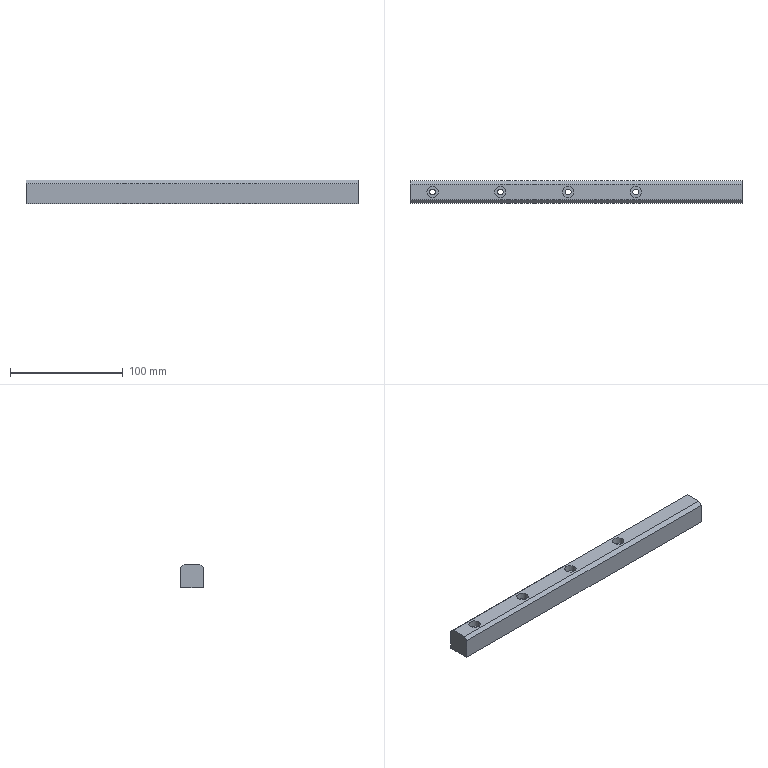Part | NX | 1 solid | 20 faces | box 294 x 20 x 21 mm | volume 117693 mm3 | plane 12 | cylinder 8 | commonest cylinder face diameters 5.3 x4 10 x4
STEP:
#1=CARTESIAN_POINT('',(-124.35,0.,0.));
#2=VERTEX_POINT('',#1);
#3=CARTESIAN_POINT('',(-127.,0.,0.));
#4=DIRECTION('',(0.,0.,1.));
#5=DIRECTION('',(1.,0.,0.));
#6=AXIS2_PLACEMENT_3D('',#3,#4,#5);
#7=CIRCLE('',#6,2.65);
#8=EDGE_CURVE('',#2,#2,#7,.T.);
#9=ORIENTED_EDGE('',*,*,#8,.F.);
#10=EDGE_LOOP('',(#9));
#11=FACE_BOUND('',#10,.T.);
#12=CARTESIAN_POINT('',(-124.35,0.,15.3));
#13=VERTEX_POINT('',#12);
#14=CARTESIAN_POINT('',(-127.,0.,15.3));
#15=DIRECTION('',(0.,0.,1.));
#16=DIRECTION('',(1.,0.,0.));
#17=AXIS2_PLACEMENT_3D('',#14,#15,#16);
#18=CIRCLE('',#17,2.65);
#19=EDGE_CURVE('',#13,#13,#18,.T.);
#20=ORIENTED_EDGE('',*,*,#19,.T.);
#21=EDGE_LOOP('',(#20));
#22=FACE_BOUND('',#21,.T.);
#23=CARTESIAN_POINT('',(-127.,0.,294.));
#24=DIRECTION('',(0.,0.,-1.));
#25=DIRECTION('',(1.,0.,0.));
#26=AXIS2_PLACEMENT_3D('',#23,#24,#25);
#27=CYLINDRICAL_SURFACE('',#26,2.65);
#28=ADVANCED_FACE('',(#11,#22),#27,.F.);
#29=CARTESIAN_POINT('',(-64.35,0.,0.));
#30=VERTEX_POINT('',#29);
#31=CARTESIAN_POINT('',(-67.,0.,0.));
#32=DIRECTION('',(0.,0.,1.));
#33=DIRECTION('',(1.,0.,0.));
#34=AXIS2_PLACEMENT_3D('',#31,#32,#33);
#35=CIRCLE('',#34,2.65);
#36=EDGE_CURVE('',#30,#30,#35,.T.);
#37=ORIENTED_EDGE('',*,*,#36,.F.);
#38=EDGE_LOOP('',(#37));
#39=FACE_BOUND('',#38,.T.);
#40=CARTESIAN_POINT('',(-64.35,0.,15.3));
#41=VERTEX_POINT('',#40);
#42=CARTESIAN_POINT('',(-67.,0.,15.3));
#43=DIRECTION('',(0.,0.,1.));
#44=DIRECTION('',(1.,0.,0.));
#45=AXIS2_PLACEMENT_3D('',#42,#43,#44);
#46=CIRCLE('',#45,2.65);
#47=EDGE_CURVE('',#41,#41,#46,.T.);
#48=ORIENTED_EDGE('',*,*,#47,.T.);
#49=EDGE_LOOP('',(#48));
#50=FACE_BOUND('',#49,.T.);
#51=CARTESIAN_POINT('',(-67.,0.,294.));
#52=DIRECTION('',(0.,0.,-1.));
#53=DIRECTION('',(1.,0.,0.));
#54=AXIS2_PLACEMENT_3D('',#51,#52,#53);
#55=CYLINDRICAL_SURFACE('',#54,2.65);
#56=ADVANCED_FACE('',(#39,#50),#55,.F.);
#57=CARTESIAN_POINT('',(-4.35,0.,0.));
#58=VERTEX_POINT('',#57);
#59=CARTESIAN_POINT('',(-7.,0.,0.));
#60=DIRECTION('',(0.,0.,1.));
#61=DIRECTION('',(1.,0.,0.));
#62=AXIS2_PLACEMENT_3D('',#59,#60,#61);
#63=CIRCLE('',#62,2.65);
#64=EDGE_CURVE('',#58,#58,#63,.T.);
#65=ORIENTED_EDGE('',*,*,#64,.F.);
#66=EDGE_LOOP('',(#65));
#67=FACE_BOUND('',#66,.T.);
#68=CARTESIAN_POINT('',(-4.35,0.,15.3));
#69=VERTEX_POINT('',#68);
#70=CARTESIAN_POINT('',(-7.,0.,15.3));
#71=DIRECTION('',(0.,0.,1.));
#72=DIRECTION('',(1.,0.,0.));
#73=AXIS2_PLACEMENT_3D('',#70,#71,#72);
#74=CIRCLE('',#73,2.65);
#75=EDGE_CURVE('',#69,#69,#74,.T.);
#76=ORIENTED_EDGE('',*,*,#75,.T.);
#77=EDGE_LOOP('',(#76));
#78=FACE_BOUND('',#77,.T.);
#79=CARTESIAN_POINT('',(-7.,0.,294.));
#80=DIRECTION('',(0.,0.,-1.));
#81=DIRECTION('',(1.,0.,0.));
#82=AXIS2_PLACEMENT_3D('',#79,#80,#81);
#83=CYLINDRICAL_SURFACE('',#82,2.65);
#84=ADVANCED_FACE('',(#67,#78),#83,.F.);
#85=CARTESIAN_POINT('',(55.65,0.,0.));
#86=VERTEX_POINT('',#85);
#87=CARTESIAN_POINT('',(53.,0.,0.));
#88=DIRECTION('',(0.,0.,1.));
#89=DIRECTION('',(1.,0.,0.));
#90=AXIS2_PLACEMENT_3D('',#87,#88,#89);
#91=CIRCLE('',#90,2.65);
#92=EDGE_CURVE('',#86,#86,#91,.T.);
#93=ORIENTED_EDGE('',*,*,#92,.F.);
#94=EDGE_LOOP('',(#93));
#95=FACE_BOUND('',#94,.T.);
#96=CARTESIAN_POINT('',(55.65,0.,15.3));
#97=VERTEX_POINT('',#96);
#98=CARTESIAN_POINT('',(53.,0.,15.3));
#99=DIRECTION('',(0.,0.,1.));
#100=DIRECTION('',(1.,0.,0.));
#101=AXIS2_PLACEMENT_3D('',#98,#99,#100);
#102=CIRCLE('',#101,2.65);
#103=EDGE_CURVE('',#97,#97,#102,.T.);
#104=ORIENTED_EDGE('',*,*,#103,.T.);
#105=EDGE_LOOP('',(#104));
#106=FACE_BOUND('',#105,.T.);
#107=CARTESIAN_POINT('',(53.,0.,294.));
#108=DIRECTION('',(0.,0.,-1.));
#109=DIRECTION('',(1.,0.,0.));
#110=AXIS2_PLACEMENT_3D('',#107,#108,#109);
#111=CYLINDRICAL_SURFACE('',#110,2.65);
#112=ADVANCED_FACE('',(#95,#106),#111,.F.);
#113=CARTESIAN_POINT('',(147.,-10.,18.));
#114=VERTEX_POINT('',#113);
#115=CARTESIAN_POINT('',(147.,-10.,0.));
#116=VERTEX_POINT('',#115);
#117=CARTESIAN_POINT('',(147.,-10.,18.));
#118=DIRECTION('',(0.,0.,-1.));
#119=VECTOR('',#118,1.);
#120=LINE('',#117,#119);
#121=EDGE_CURVE('',#114,#116,#120,.T.);
#122=ORIENTED_EDGE('',*,*,#121,.F.);
#123=CARTESIAN_POINT('',(-147.,-10.,18.));
#124=VERTEX_POINT('',#123);
#125=CARTESIAN_POINT('',(-147.,-10.,18.));
#126=DIRECTION('',(1.,0.,0.));
#127=VECTOR('',#126,1.);
#128=LINE('',#125,#127);
#129=EDGE_CURVE('',#124,#114,#128,.T.);
#130=ORIENTED_EDGE('',*,*,#129,.F.);
#131=CARTESIAN_POINT('',(-147.,-10.,0.));
#132=VERTEX_POINT('',#131);
#133=CARTESIAN_POINT('',(-147.,-10.,18.));
#134=DIRECTION('',(0.,0.,-1.));
#135=VECTOR('',#134,1.);
#136=LINE('',#133,#135);
#137=EDGE_CURVE('',#124,#132,#136,.T.);
#138=ORIENTED_EDGE('',*,*,#137,.T.);
#139=CARTESIAN_POINT('',(-147.,-10.,0.));
#140=DIRECTION('',(1.,0.,0.));
#141=VECTOR('',#140,1.);
#142=LINE('',#139,#141);
#143=EDGE_CURVE('',#132,#116,#142,.T.);
#144=ORIENTED_EDGE('',*,*,#143,.T.);
#145=EDGE_LOOP('',(#122,#130,#138,#144));
#146=FACE_OUTER_BOUND('',#145,.T.);
#147=CARTESIAN_POINT('',(-147.,-10.,18.));
#148=DIRECTION('',(0.,-1.,0.));
#149=DIRECTION('',(0.,0.,1.));
#150=AXIS2_PLACEMENT_3D('',#147,#148,#149);
#151=PLANE('',#150);
#152=ADVANCED_FACE('',(#146),#151,.T.);
#153=ORIENTED_EDGE('',*,*,#92,.T.);
#154=EDGE_LOOP('',(#153));
#155=FACE_BOUND('',#154,.T.);
#156=ORIENTED_EDGE('',*,*,#64,.T.);
#157=EDGE_LOOP('',(#156));
#158=FACE_BOUND('',#157,.T.);
#159=ORIENTED_EDGE('',*,*,#36,.T.);
#160=EDGE_LOOP('',(#159));
#161=FACE_BOUND('',#160,.T.);
#162=ORIENTED_EDGE('',*,*,#8,.T.);
#163=EDGE_LOOP('',(#162));
#164=FACE_BOUND('',#163,.T.);
#165=CARTESIAN_POINT('',(147.,10.,0.));
#166=VERTEX_POINT('',#165);
#167=CARTESIAN_POINT('',(147.,-10.,0.));
#168=DIRECTION('',(0.,1.,0.));
#169=VECTOR('',#168,1.);
#170=LINE('',#167,#169);
#171=EDGE_CURVE('',#116,#166,#170,.T.);
#172=ORIENTED_EDGE('',*,*,#171,.F.);
#173=ORIENTED_EDGE('',*,*,#143,.F.);
#174=CARTESIAN_POINT('',(-147.,10.,0.));
#175=VERTEX_POINT('',#174);
#176=CARTESIAN_POINT('',(-147.,-10.,0.));
#177=DIRECTION('',(0.,1.,0.));
#178=VECTOR('',#177,1.);
#179=LINE('',#176,#178);
#180=EDGE_CURVE('',#132,#175,#179,.T.);
#181=ORIENTED_EDGE('',*,*,#180,.T.);
#182=CARTESIAN_POINT('',(-147.,10.,0.));
#183=DIRECTION('',(1.,0.,0.));
#184=VECTOR('',#183,1.);
#185=LINE('',#182,#184);
#186=EDGE_CURVE('',#175,#166,#185,.T.);
#187=ORIENTED_EDGE('',*,*,#186,.T.);
#188=EDGE_LOOP('',(#172,#173,#181,#187));
#189=FACE_BOUND('',#188,.T.);
#190=CARTESIAN_POINT('',(-147.,-10.,0.));
#191=DIRECTION('',(0.,0.,-1.));
#192=DIRECTION('',(1.,0.,0.));
#193=AXIS2_PLACEMENT_3D('',#190,#191,#192);
#194=PLANE('',#193);
#195=ADVANCED_FACE('',(#155,#158,#161,#164,#189),#194,.T.);
#196=CARTESIAN_POINT('',(147.,10.,18.));
#197=VERTEX_POINT('',#196);
#198=CARTESIAN_POINT('',(147.,10.,0.));
#199=DIRECTION('',(0.,0.,1.));
#200=VECTOR('',#199,1.);
#201=LINE('',#198,#200);
#202=EDGE_CURVE('',#166,#197,#201,.T.);
#203=ORIENTED_EDGE('',*,*,#202,.F.);
#204=ORIENTED_EDGE('',*,*,#186,.F.);
#205=CARTESIAN_POINT('',(-147.,10.,18.));
#206=VERTEX_POINT('',#205);
#207=CARTESIAN_POINT('',(-147.,10.,0.));
#208=DIRECTION('',(0.,0.,1.));
#209=VECTOR('',#208,1.);
#210=LINE('',#207,#209);
#211=EDGE_CURVE('',#175,#206,#210,.T.);
#212=ORIENTED_EDGE('',*,*,#211,.T.);
#213=CARTESIAN_POINT('',(-147.,10.,18.));
#214=DIRECTION('',(1.,0.,0.));
#215=VECTOR('',#214,1.);
#216=LINE('',#213,#215);
#217=EDGE_CURVE('',#206,#197,#216,.T.);
#218=ORIENTED_EDGE('',*,*,#217,.T.);
#219=EDGE_LOOP('',(#203,#204,#212,#218));
#220=FACE_OUTER_BOUND('',#219,.T.);
#221=CARTESIAN_POINT('',(-147.,10.,0.));
#222=DIRECTION('',(0.,1.,0.));
#223=DIRECTION('',(0.,0.,-1.));
#224=AXIS2_PLACEMENT_3D('',#221,#222,#223);
#225=PLANE('',#224);
#226=ADVANCED_FACE('',(#220),#225,.T.);
#227=CARTESIAN_POINT('',(147.,7.,21.));
#228=VERTEX_POINT('',#227);
#229=CARTESIAN_POINT('',(147.,10.,18.));
#230=DIRECTION('',(0.,-0.7071,0.7071));
#231=VECTOR('',#230,1.);
#232=LINE('',#229,#231);
#233=EDGE_CURVE('',#197,#228,#232,.T.);
#234=ORIENTED_EDGE('',*,*,#233,.F.);
#235=ORIENTED_EDGE('',*,*,#217,.F.);
#236=CARTESIAN_POINT('',(-147.,7.,21.));
#237=VERTEX_POINT('',#236);
#238=CARTESIAN_POINT('',(-147.,10.,18.));
#239=DIRECTION('',(0.,-0.7071,0.7071));
#240=VECTOR('',#239,1.);
#241=LINE('',#238,#240);
#242=EDGE_CURVE('',#206,#237,#241,.T.);
#243=ORIENTED_EDGE('',*,*,#242,.T.);
#244=CARTESIAN_POINT('',(-147.,7.,21.));
#245=DIRECTION('',(1.,0.,0.));
#246=VECTOR('',#245,1.);
#247=LINE('',#244,#246);
#248=EDGE_CURVE('',#237,#228,#247,.T.);
#249=ORIENTED_EDGE('',*,*,#248,.T.);
#250=EDGE_LOOP('',(#234,#235,#243,#249));
#251=FACE_OUTER_BOUND('',#250,.T.);
#252=CARTESIAN_POINT('',(-147.,10.,18.));
#253=DIRECTION('',(0.,0.7071,0.7071));
#254=DIRECTION('',(0.,0.7071,-0.7071));
#255=AXIS2_PLACEMENT_3D('',#252,#253,#254);
#256=PLANE('',#255);
#257=ADVANCED_FACE('',(#251),#256,.T.);
#258=CARTESIAN_POINT('',(58.,0.,21.));
#259=VERTEX_POINT('',#258);
#260=CARTESIAN_POINT('',(53.,0.,21.));
#261=DIRECTION('',(0.,0.,-1.));
#262=DIRECTION('',(1.,0.,0.));
#263=AXIS2_PLACEMENT_3D('',#260,#261,#262);
#264=CIRCLE('',#263,5.);
#265=EDGE_CURVE('',#259,#259,#264,.T.);
#266=ORIENTED_EDGE('',*,*,#265,.T.);
#267=EDGE_LOOP('',(#266));
#268=FACE_BOUND('',#267,.T.);
#269=CARTESIAN_POINT('',(-2.,0.,21.));
#270=VERTEX_POINT('',#269);
#271=CARTESIAN_POINT('',(-7.,0.,21.));
#272=DIRECTION('',(0.,0.,-1.));
#273=DIRECTION('',(1.,0.,0.));
#274=AXIS2_PLACEMENT_3D('',#271,#272,#273);
#275=CIRCLE('',#274,5.);
#276=EDGE_CURVE('',#270,#270,#275,.T.);
#277=ORIENTED_EDGE('',*,*,#276,.T.);
#278=EDGE_LOOP('',(#277));
#279=FACE_BOUND('',#278,.T.);
#280=CARTESIAN_POINT('',(-62.,0.,21.));
#281=VERTEX_POINT('',#280);
#282=CARTESIAN_POINT('',(-67.,0.,21.));
#283=DIRECTION('',(0.,0.,-1.));
#284=DIRECTION('',(1.,0.,0.));
#285=AXIS2_PLACEMENT_3D('',#282,#283,#284);
#286=CIRCLE('',#285,5.);
#287=EDGE_CURVE('',#281,#281,#286,.T.);
#288=ORIENTED_EDGE('',*,*,#287,.T.);
#289=EDGE_LOOP('',(#288));
#290=FACE_BOUND('',#289,.T.);
#291=CARTESIAN_POINT('',(-122.,0.,21.));
#292=VERTEX_POINT('',#291);
#293=CARTESIAN_POINT('',(-127.,0.,21.));
#294=DIRECTION('',(0.,0.,-1.));
#295=DIRECTION('',(1.,0.,0.));
#296=AXIS2_PLACEMENT_3D('',#293,#294,#295);
#297=CIRCLE('',#296,5.);
#298=EDGE_CURVE('',#292,#292,#297,.T.);
#299=ORIENTED_EDGE('',*,*,#298,.T.);
#300=EDGE_LOOP('',(#299));
#301=FACE_BOUND('',#300,.T.);
#302=CARTESIAN_POINT('',(147.,-7.,21.));
#303=VERTEX_POINT('',#302);
#304=CARTESIAN_POINT('',(147.,7.,21.));
#305=DIRECTION('',(0.,-1.,0.));
#306=VECTOR('',#305,1.);
#307=LINE('',#304,#306);
#308=EDGE_CURVE('',#228,#303,#307,.T.);
#309=ORIENTED_EDGE('',*,*,#308,.F.);
#310=ORIENTED_EDGE('',*,*,#248,.F.);
#311=CARTESIAN_POINT('',(-147.,-7.,21.));
#312=VERTEX_POINT('',#311);
#313=CARTESIAN_POINT('',(-147.,7.,21.));
#314=DIRECTION('',(0.,-1.,0.));
#315=VECTOR('',#314,1.);
#316=LINE('',#313,#315);
#317=EDGE_CURVE('',#237,#312,#316,.T.);
#318=ORIENTED_EDGE('',*,*,#317,.T.);
#319=CARTESIAN_POINT('',(-147.,-7.,21.));
#320=DIRECTION('',(1.,0.,0.));
#321=VECTOR('',#320,1.);
#322=LINE('',#319,#321);
#323=EDGE_CURVE('',#312,#303,#322,.T.);
#324=ORIENTED_EDGE('',*,*,#323,.T.);
#325=EDGE_LOOP('',(#309,#310,#318,#324));
#326=FACE_BOUND('',#325,.T.);
#327=CARTESIAN_POINT('',(-147.,7.,21.));
#328=DIRECTION('',(0.,0.,1.));
#329=DIRECTION('',(-1.,0.,0.));
#330=AXIS2_PLACEMENT_3D('',#327,#328,#329);
#331=PLANE('',#330);
#332=ADVANCED_FACE('',(#268,#279,#290,#301,#326),#331,.T.);
#333=CARTESIAN_POINT('',(147.,-7.,21.));
#334=DIRECTION('',(0.,-0.7071,-0.7071));
#335=VECTOR('',#334,1.);
#336=LINE('',#333,#335);
#337=EDGE_CURVE('',#303,#114,#336,.T.);
#338=ORIENTED_EDGE('',*,*,#337,.F.);
#339=ORIENTED_EDGE('',*,*,#323,.F.);
#340=CARTESIAN_POINT('',(-147.,-7.,21.));
#341=DIRECTION('',(0.,-0.7071,-0.7071));
#342=VECTOR('',#341,1.);
#343=LINE('',#340,#342);
#344=EDGE_CURVE('',#312,#124,#343,.T.);
#345=ORIENTED_EDGE('',*,*,#344,.T.);
#346=ORIENTED_EDGE('',*,*,#129,.T.);
#347=EDGE_LOOP('',(#338,#339,#345,#346));
#348=FACE_OUTER_BOUND('',#347,.T.);
#349=CARTESIAN_POINT('',(-147.,-7.,21.));
#350=DIRECTION('',(0.,-0.7071,0.7071));
#351=DIRECTION('',(0.,0.7071,0.7071));
#352=AXIS2_PLACEMENT_3D('',#349,#350,#351);
#353=PLANE('',#352);
#354=ADVANCED_FACE('',(#348),#353,.T.);
#355=ORIENTED_EDGE('',*,*,#137,.F.);
#356=ORIENTED_EDGE('',*,*,#344,.F.);
#357=ORIENTED_EDGE('',*,*,#317,.F.);
#358=ORIENTED_EDGE('',*,*,#242,.F.);
#359=ORIENTED_EDGE('',*,*,#211,.F.);
#360=ORIENTED_EDGE('',*,*,#180,.F.);
#361=EDGE_LOOP('',(#355,#356,#357,#358,#359,#360));
#362=FACE_OUTER_BOUND('',#361,.T.);
#363=CARTESIAN_POINT('',(-147.,0.,0.));
#364=DIRECTION('',(1.,0.,0.));
#365=DIRECTION('',(0.,0.,1.));
#366=AXIS2_PLACEMENT_3D('',#363,#364,#365);
#367=PLANE('',#366);
#368=ADVANCED_FACE('',(#362),#367,.F.);
#369=ORIENTED_EDGE('',*,*,#121,.T.);
#370=ORIENTED_EDGE('',*,*,#171,.T.);
#371=ORIENTED_EDGE('',*,*,#202,.T.);
#372=ORIENTED_EDGE('',*,*,#233,.T.);
#373=ORIENTED_EDGE('',*,*,#308,.T.);
#374=ORIENTED_EDGE('',*,*,#337,.T.);
#375=EDGE_LOOP('',(#369,#370,#371,#372,#373,#374));
#376=FACE_OUTER_BOUND('',#375,.T.);
#377=CARTESIAN_POINT('',(147.,0.,0.));
#378=DIRECTION('',(1.,0.,0.));
#379=DIRECTION('',(0.,0.,1.));
#380=AXIS2_PLACEMENT_3D('',#377,#378,#379);
#381=PLANE('',#380);
#382=ADVANCED_FACE('',(#376),#381,.T.);
#383=ORIENTED_EDGE('',*,*,#265,.F.);
#384=EDGE_LOOP('',(#383));
#385=FACE_BOUND('',#384,.T.);
#386=CARTESIAN_POINT('',(58.,0.,15.3));
#387=VERTEX_POINT('',#386);
#388=CARTESIAN_POINT('',(53.,0.,15.3));
#389=DIRECTION('',(0.,0.,-1.));
#390=DIRECTION('',(1.,0.,0.));
#391=AXIS2_PLACEMENT_3D('',#388,#389,#390);
#392=CIRCLE('',#391,5.);
#393=EDGE_CURVE('',#387,#387,#392,.T.);
#394=ORIENTED_EDGE('',*,*,#393,.T.);
#395=EDGE_LOOP('',(#394));
#396=FACE_BOUND('',#395,.T.);
#397=CARTESIAN_POINT('',(53.,0.,294.));
#398=DIRECTION('',(0.,0.,-1.));
#399=DIRECTION('',(1.,0.,0.));
#400=AXIS2_PLACEMENT_3D('',#397,#398,#399);
#401=CYLINDRICAL_SURFACE('',#400,5.);
#402=ADVANCED_FACE('',(#385,#396),#401,.F.);
#403=ORIENTED_EDGE('',*,*,#103,.F.);
#404=EDGE_LOOP('',(#403));
#405=FACE_BOUND('',#404,.T.);
#406=ORIENTED_EDGE('',*,*,#393,.F.);
#407=EDGE_LOOP('',(#406));
#408=FACE_BOUND('',#407,.T.);
#409=CARTESIAN_POINT('',(53.,0.,15.3));
#410=DIRECTION('',(0.,0.,1.));
#411=DIRECTION('',(-1.,0.,0.));
#412=AXIS2_PLACEMENT_3D('',#409,#410,#411);
#413=PLANE('',#412);
#414=ADVANCED_FACE('',(#405,#408),#413,.T.);
#415=ORIENTED_EDGE('',*,*,#276,.F.);
#416=EDGE_LOOP('',(#415));
#417=FACE_BOUND('',#416,.T.);
#418=CARTESIAN_POINT('',(-2.,0.,15.3));
#419=VERTEX_POINT('',#418);
#420=CARTESIAN_POINT('',(-7.,0.,15.3));
#421=DIRECTION('',(0.,0.,-1.));
#422=DIRECTION('',(1.,0.,0.));
#423=AXIS2_PLACEMENT_3D('',#420,#421,#422);
#424=CIRCLE('',#423,5.);
#425=EDGE_CURVE('',#419,#419,#424,.T.);
#426=ORIENTED_EDGE('',*,*,#425,.T.);
#427=EDGE_LOOP('',(#426));
#428=FACE_BOUND('',#427,.T.);
#429=CARTESIAN_POINT('',(-7.,0.,294.));
#430=DIRECTION('',(0.,0.,-1.));
#431=DIRECTION('',(1.,0.,0.));
#432=AXIS2_PLACEMENT_3D('',#429,#430,#431);
#433=CYLINDRICAL_SURFACE('',#432,5.);
#434=ADVANCED_FACE('',(#417,#428),#433,.F.);
#435=ORIENTED_EDGE('',*,*,#75,.F.);
#436=EDGE_LOOP('',(#435));
#437=FACE_BOUND('',#436,.T.);
#438=ORIENTED_EDGE('',*,*,#425,.F.);
#439=EDGE_LOOP('',(#438));
#440=FACE_BOUND('',#439,.T.);
#441=CARTESIAN_POINT('',(-7.,0.,15.3));
#442=DIRECTION('',(0.,0.,1.));
#443=DIRECTION('',(-1.,0.,0.));
#444=AXIS2_PLACEMENT_3D('',#441,#442,#443);
#445=PLANE('',#444);
#446=ADVANCED_FACE('',(#437,#440),#445,.T.);
#447=ORIENTED_EDGE('',*,*,#287,.F.);
#448=EDGE_LOOP('',(#447));
#449=FACE_BOUND('',#448,.T.);
#450=CARTESIAN_POINT('',(-62.,0.,15.3));
#451=VERTEX_POINT('',#450);
#452=CARTESIAN_POINT('',(-67.,0.,15.3));
#453=DIRECTION('',(0.,0.,-1.));
#454=DIRECTION('',(1.,0.,0.));
#455=AXIS2_PLACEMENT_3D('',#452,#453,#454);
#456=CIRCLE('',#455,5.);
#457=EDGE_CURVE('',#451,#451,#456,.T.);
#458=ORIENTED_EDGE('',*,*,#457,.T.);
#459=EDGE_LOOP('',(#458));
#460=FACE_BOUND('',#459,.T.);
#461=CARTESIAN_POINT('',(-67.,0.,294.));
#462=DIRECTION('',(0.,0.,-1.));
#463=DIRECTION('',(1.,0.,0.));
#464=AXIS2_PLACEMENT_3D('',#461,#462,#463);
#465=CYLINDRICAL_SURFACE('',#464,5.);
#466=ADVANCED_FACE('',(#449,#460),#465,.F.);
#467=ORIENTED_EDGE('',*,*,#47,.F.);
#468=EDGE_LOOP('',(#467));
#469=FACE_BOUND('',#468,.T.);
#470=ORIENTED_EDGE('',*,*,#457,.F.);
#471=EDGE_LOOP('',(#470));
#472=FACE_BOUND('',#471,.T.);
#473=CARTESIAN_POINT('',(-67.,0.,15.3));
#474=DIRECTION('',(0.,0.,1.));
#475=DIRECTION('',(-1.,0.,0.));
#476=AXIS2_PLACEMENT_3D('',#473,#474,#475);
#477=PLANE('',#476);
#478=ADVANCED_FACE('',(#469,#472),#477,.T.);
#479=ORIENTED_EDGE('',*,*,#298,.F.);
#480=EDGE_LOOP('',(#479));
#481=FACE_BOUND('',#480,.T.);
#482=CARTESIAN_POINT('',(-122.,0.,15.3));
#483=VERTEX_POINT('',#482);
#484=CARTESIAN_POINT('',(-127.,0.,15.3));
#485=DIRECTION('',(0.,0.,-1.));
#486=DIRECTION('',(1.,0.,0.));
#487=AXIS2_PLACEMENT_3D('',#484,#485,#486);
#488=CIRCLE('',#487,5.);
#489=EDGE_CURVE('',#483,#483,#488,.T.);
#490=ORIENTED_EDGE('',*,*,#489,.T.);
#491=EDGE_LOOP('',(#490));
#492=FACE_BOUND('',#491,.T.);
#493=CARTESIAN_POINT('',(-127.,0.,294.));
#494=DIRECTION('',(0.,0.,-1.));
#495=DIRECTION('',(1.,0.,0.));
#496=AXIS2_PLACEMENT_3D('',#493,#494,#495);
#497=CYLINDRICAL_SURFACE('',#496,5.);
#498=ADVANCED_FACE('',(#481,#492),#497,.F.);
#499=ORIENTED_EDGE('',*,*,#19,.F.);
#500=EDGE_LOOP('',(#499));
#501=FACE_BOUND('',#500,.T.);
#502=ORIENTED_EDGE('',*,*,#489,.F.);
#503=EDGE_LOOP('',(#502));
#504=FACE_BOUND('',#503,.T.);
#505=CARTESIAN_POINT('',(-127.,0.,15.3));
#506=DIRECTION('',(0.,0.,1.));
#507=DIRECTION('',(-1.,0.,0.));
#508=AXIS2_PLACEMENT_3D('',#505,#506,#507);
#509=PLANE('',#508);
#510=ADVANCED_FACE('',(#501,#504),#509,.T.);
#511=CLOSED_SHELL('',(#28,#56,#84,#112,#152,#195,#226,#257,#332,#354,#368,#382,#402,#414,#434,#446,#466,#478,#498,#510));
#512=MANIFOLD_SOLID_BREP('',#511);
#513=(LENGTH_UNIT()NAMED_UNIT(*)SI_UNIT(.MILLI.,.METRE.));
#514=UNCERTAINTY_MEASURE_WITH_UNIT(LENGTH_MEASURE(0.00002),#513,'','');
#515=(NAMED_UNIT(*)PLANE_ANGLE_UNIT()SI_UNIT($,.RADIAN.));
#516=PLANE_ANGLE_MEASURE_WITH_UNIT(PLANE_ANGLE_MEASURE(0.01745),#515);
#517=DIMENSIONAL_EXPONENTS(0.,0.,0.,0.,0.,0.,0.);
#518=(CONVERSION_BASED_UNIT('DEGREE',#516)NAMED_UNIT(#517)PLANE_ANGLE_UNIT());
#519=(NAMED_UNIT(*)SI_UNIT($,.STERADIAN.)SOLID_ANGLE_UNIT());
#520=(GEOMETRIC_REPRESENTATION_CONTEXT(3)GLOBAL_UNCERTAINTY_ASSIGNED_CONTEXT((#514))GLOBAL_UNIT_ASSIGNED_CONTEXT((#513,#518,#519))REPRESENTATION_CONTEXT('',''));
#521=ADVANCED_BREP_SHAPE_REPRESENTATION('',(#512),#520);